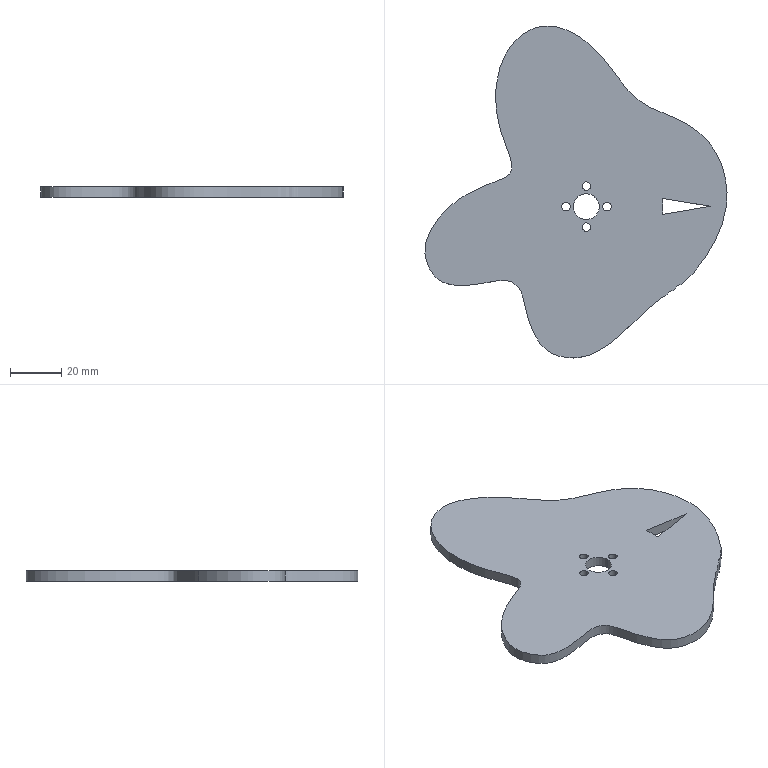Part | SolidWorks | features CurveInFile 1, Extrusion 1 | 1 solid | 18 faces | box 117.822 x 129.451 x 4 mm | volume 34423 mm3 | cylinder 10 | plane 6 | spline 2 | commonest cylinder face diameters 3.3 x8 10.1 x2